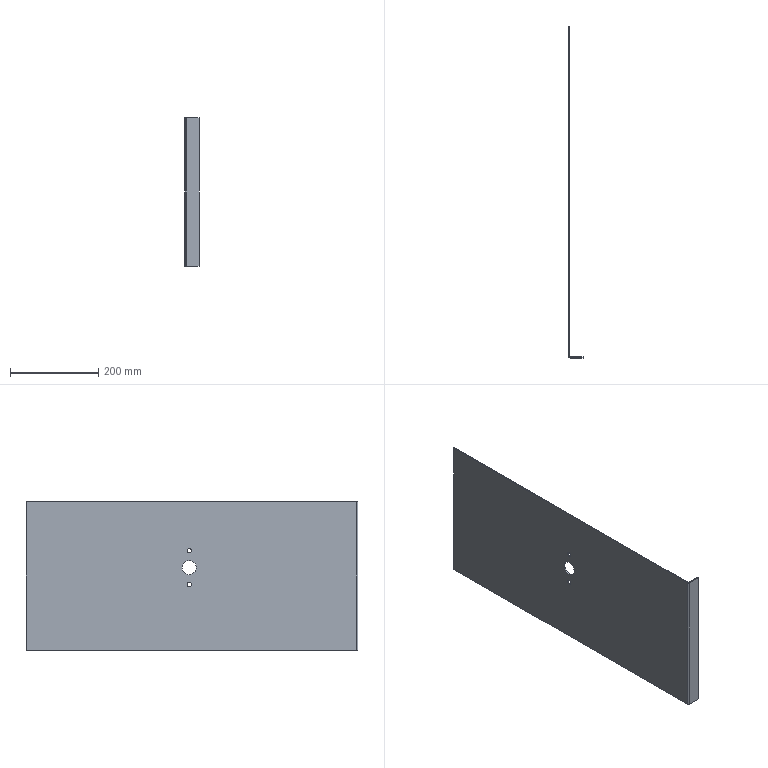Part | SolidWorks | features FlatPattern 1, ICE 1, SMBaseFlange 1, SheetMetal 1 | 1 solid | 20 faces | box 32 x 752 x 337 mm | volume 524643 mm3 | plane 12 | cylinder 8 | commonest cylinder face diameters 10 x4 32 x2 1.473 x1 5.473 x1
STEP:
#1=CARTESIAN_POINT('',(0.,107.626,-14.25));
#2=VERTEX_POINT('',#1);
#3=CARTESIAN_POINT('',(0.,107.626,-24.25));
#4=VERTEX_POINT('',#3);
#5=CARTESIAN_POINT('',(0.,107.626,-19.25));
#6=DIRECTION('',(1.,0.,0.));
#7=DIRECTION('',(0.,0.,-1.));
#8=AXIS2_PLACEMENT_3D('',#5,#6,#7);
#9=CIRCLE('',#8,5.);
#10=EDGE_CURVE('',#2,#4,#9,.T.);
#11=ORIENTED_EDGE('',*,*,#10,.T.);
#12=CARTESIAN_POINT('',(-2.,107.626,-24.25));
#13=VERTEX_POINT('',#12);
#14=CARTESIAN_POINT('',(8.,107.626,-24.25));
#15=DIRECTION('',(-1.,0.,0.));
#16=VECTOR('',#15,1000.);
#17=LINE('',#14,#16);
#18=EDGE_CURVE('',#4,#13,#17,.T.);
#19=ORIENTED_EDGE('',*,*,#18,.T.);
#20=CARTESIAN_POINT('',(-2.,107.626,-14.25));
#21=VERTEX_POINT('',#20);
#22=CARTESIAN_POINT('',(-2.,107.626,-19.25));
#23=DIRECTION('',(-1.,0.,0.));
#24=DIRECTION('',(0.,0.,1.));
#25=AXIS2_PLACEMENT_3D('',#22,#23,#24);
#26=CIRCLE('',#25,5.);
#27=EDGE_CURVE('',#13,#21,#26,.T.);
#28=ORIENTED_EDGE('',*,*,#27,.T.);
#29=CARTESIAN_POINT('',(8.,107.626,-14.25));
#30=DIRECTION('',(-1.,0.,0.));
#31=VECTOR('',#30,1000.);
#32=LINE('',#29,#31);
#33=EDGE_CURVE('',#2,#21,#32,.T.);
#34=ORIENTED_EDGE('',*,*,#33,.F.);
#35=EDGE_LOOP('',(#11,#19,#28,#34));
#36=FACE_OUTER_BOUND('',#35,.T.);
#37=CARTESIAN_POINT('',(8.,107.626,-19.25));
#38=DIRECTION('',(-1.,0.,0.));
#39=DIRECTION('',(0.,0.,1.));
#40=AXIS2_PLACEMENT_3D('',#37,#38,#39);
#41=CYLINDRICAL_SURFACE('',#40,5.);
#42=ADVANCED_FACE('',(#36),#41,.F.);
#43=CARTESIAN_POINT('',(0.,107.626,62.25));
#44=VERTEX_POINT('',#43);
#45=CARTESIAN_POINT('',(0.,107.626,52.25));
#46=VERTEX_POINT('',#45);
#47=CARTESIAN_POINT('',(0.,107.626,57.25));
#48=DIRECTION('',(1.,0.,0.));
#49=DIRECTION('',(0.,0.,-1.));
#50=AXIS2_PLACEMENT_3D('',#47,#48,#49);
#51=CIRCLE('',#50,5.);
#52=EDGE_CURVE('',#44,#46,#51,.T.);
#53=ORIENTED_EDGE('',*,*,#52,.T.);
#54=CARTESIAN_POINT('',(-2.,107.626,52.25));
#55=VERTEX_POINT('',#54);
#56=CARTESIAN_POINT('',(8.,107.626,52.25));
#57=DIRECTION('',(-1.,0.,0.));
#58=VECTOR('',#57,1000.);
#59=LINE('',#56,#58);
#60=EDGE_CURVE('',#46,#55,#59,.T.);
#61=ORIENTED_EDGE('',*,*,#60,.T.);
#62=CARTESIAN_POINT('',(-2.,107.626,62.25));
#63=VERTEX_POINT('',#62);
#64=CARTESIAN_POINT('',(-2.,107.626,57.25));
#65=DIRECTION('',(-1.,0.,0.));
#66=DIRECTION('',(0.,0.,1.));
#67=AXIS2_PLACEMENT_3D('',#64,#65,#66);
#68=CIRCLE('',#67,5.);
#69=EDGE_CURVE('',#55,#63,#68,.T.);
#70=ORIENTED_EDGE('',*,*,#69,.T.);
#71=CARTESIAN_POINT('',(8.,107.626,62.25));
#72=DIRECTION('',(-1.,0.,0.));
#73=VECTOR('',#72,1000.);
#74=LINE('',#71,#73);
#75=EDGE_CURVE('',#44,#63,#74,.T.);
#76=ORIENTED_EDGE('',*,*,#75,.F.);
#77=EDGE_LOOP('',(#53,#61,#70,#76));
#78=FACE_OUTER_BOUND('',#77,.T.);
#79=CARTESIAN_POINT('',(8.,107.626,57.25));
#80=DIRECTION('',(-1.,0.,0.));
#81=DIRECTION('',(0.,0.,1.));
#82=AXIS2_PLACEMENT_3D('',#79,#80,#81);
#83=CYLINDRICAL_SURFACE('',#82,5.);
#84=ADVANCED_FACE('',(#78),#83,.F.);
#85=CARTESIAN_POINT('',(0.,107.626,35.));
#86=VERTEX_POINT('',#85);
#87=CARTESIAN_POINT('',(0.,107.626,3.));
#88=VERTEX_POINT('',#87);
#89=CARTESIAN_POINT('',(0.,107.626,19.));
#90=DIRECTION('',(1.,0.,0.));
#91=DIRECTION('',(0.,0.,-1.));
#92=AXIS2_PLACEMENT_3D('',#89,#90,#91);
#93=CIRCLE('',#92,16.);
#94=EDGE_CURVE('',#86,#88,#93,.T.);
#95=ORIENTED_EDGE('',*,*,#94,.T.);
#96=CARTESIAN_POINT('',(-2.,107.626,3.));
#97=VERTEX_POINT('',#96);
#98=CARTESIAN_POINT('',(8.,107.626,3.));
#99=DIRECTION('',(-1.,0.,0.));
#100=VECTOR('',#99,1000.);
#101=LINE('',#98,#100);
#102=EDGE_CURVE('',#88,#97,#101,.T.);
#103=ORIENTED_EDGE('',*,*,#102,.T.);
#104=CARTESIAN_POINT('',(-2.,107.626,35.));
#105=VERTEX_POINT('',#104);
#106=CARTESIAN_POINT('',(-2.,107.626,19.));
#107=DIRECTION('',(-1.,0.,0.));
#108=DIRECTION('',(0.,0.,1.));
#109=AXIS2_PLACEMENT_3D('',#106,#107,#108);
#110=CIRCLE('',#109,16.);
#111=EDGE_CURVE('',#97,#105,#110,.T.);
#112=ORIENTED_EDGE('',*,*,#111,.T.);
#113=CARTESIAN_POINT('',(8.,107.626,35.));
#114=DIRECTION('',(-1.,0.,0.));
#115=VECTOR('',#114,1000.);
#116=LINE('',#113,#115);
#117=EDGE_CURVE('',#86,#105,#116,.T.);
#118=ORIENTED_EDGE('',*,*,#117,.F.);
#119=EDGE_LOOP('',(#95,#103,#112,#118));
#120=FACE_OUTER_BOUND('',#119,.T.);
#121=CARTESIAN_POINT('',(8.,107.626,19.));
#122=DIRECTION('',(-1.,0.,0.));
#123=DIRECTION('',(0.,0.,1.));
#124=AXIS2_PLACEMENT_3D('',#121,#122,#123);
#125=CYLINDRICAL_SURFACE('',#124,16.);
#126=ADVANCED_FACE('',(#120),#125,.F.);
#127=CARTESIAN_POINT('',(0.7366,-272.664,168.5));
#128=VERTEX_POINT('',#127);
#129=CARTESIAN_POINT('',(0.7366,-274.664,168.5));
#130=VERTEX_POINT('',#129);
#131=CARTESIAN_POINT('',(0.7366,-272.664,168.5));
#132=DIRECTION('',(0.,-1.,0.));
#133=VECTOR('',#132,1000.);
#134=LINE('',#131,#133);
#135=EDGE_CURVE('',#128,#130,#134,.T.);
#136=ORIENTED_EDGE('',*,*,#135,.F.);
#137=CARTESIAN_POINT('',(0.,-271.928,168.5));
#138=VERTEX_POINT('',#137);
#139=CARTESIAN_POINT('',(0.7366,-271.928,168.5));
#140=DIRECTION('',(0.,0.,1.));
#141=DIRECTION('',(-1.,0.,0.));
#142=AXIS2_PLACEMENT_3D('',#139,#140,#141);
#143=CIRCLE('',#142,0.7366);
#144=EDGE_CURVE('',#138,#128,#143,.T.);
#145=ORIENTED_EDGE('',*,*,#144,.F.);
#146=CARTESIAN_POINT('',(-2.,-271.928,168.5));
#147=VERTEX_POINT('',#146);
#148=CARTESIAN_POINT('',(-2.,-271.928,168.5));
#149=DIRECTION('',(1.,0.,0.));
#150=VECTOR('',#149,1000.);
#151=LINE('',#148,#150);
#152=EDGE_CURVE('',#147,#138,#151,.T.);
#153=ORIENTED_EDGE('',*,*,#152,.F.);
#154=CARTESIAN_POINT('',(0.7366,-271.928,168.5));
#155=DIRECTION('',(0.,0.,1.));
#156=DIRECTION('',(1.,0.,0.));
#157=AXIS2_PLACEMENT_3D('',#154,#155,#156);
#158=CIRCLE('',#157,2.737);
#159=EDGE_CURVE('',#147,#130,#158,.T.);
#160=ORIENTED_EDGE('',*,*,#159,.T.);
#161=EDGE_LOOP('',(#136,#145,#153,#160));
#162=FACE_OUTER_BOUND('',#161,.T.);
#163=CARTESIAN_POINT('',(0.7366,-272.664,168.5));
#164=DIRECTION('',(0.,0.,1.));
#165=DIRECTION('',(1.,0.,0.));
#166=AXIS2_PLACEMENT_3D('',#163,#164,#165);
#167=PLANE('',#166);
#168=ADVANCED_FACE('',(#162),#167,.T.);
#169=CARTESIAN_POINT('',(30.,-272.664,168.5));
#170=VERTEX_POINT('',#169);
#171=CARTESIAN_POINT('',(0.,-272.664,168.5));
#172=DIRECTION('',(1.,0.,0.));
#173=VECTOR('',#172,1000.);
#174=LINE('',#171,#173);
#175=EDGE_CURVE('',#128,#170,#174,.T.);
#176=ORIENTED_EDGE('',*,*,#175,.F.);
#177=ORIENTED_EDGE('',*,*,#135,.T.);
#178=CARTESIAN_POINT('',(30.,-274.664,168.5));
#179=VERTEX_POINT('',#178);
#180=CARTESIAN_POINT('',(0.,-274.664,168.5));
#181=DIRECTION('',(1.,0.,0.));
#182=VECTOR('',#181,1000.);
#183=LINE('',#180,#182);
#184=EDGE_CURVE('',#130,#179,#183,.T.);
#185=ORIENTED_EDGE('',*,*,#184,.T.);
#186=CARTESIAN_POINT('',(30.,-272.664,168.5));
#187=DIRECTION('',(0.,-1.,0.));
#188=VECTOR('',#187,1000.);
#189=LINE('',#186,#188);
#190=EDGE_CURVE('',#170,#179,#189,.T.);
#191=ORIENTED_EDGE('',*,*,#190,.F.);
#192=EDGE_LOOP('',(#176,#177,#185,#191));
#193=FACE_OUTER_BOUND('',#192,.T.);
#194=CARTESIAN_POINT('',(-2.,-271.928,168.5));
#195=DIRECTION('',(0.,0.,1.));
#196=DIRECTION('',(1.,0.,0.));
#197=AXIS2_PLACEMENT_3D('',#194,#195,#196);
#198=PLANE('',#197);
#199=ADVANCED_FACE('',(#193),#198,.T.);
#200=CARTESIAN_POINT('',(0.,-271.928,-168.5));
#201=VERTEX_POINT('',#200);
#202=CARTESIAN_POINT('',(-2.,-271.928,-168.5));
#203=VERTEX_POINT('',#202);
#204=CARTESIAN_POINT('',(0.,-271.928,-168.5));
#205=DIRECTION('',(-1.,0.,0.));
#206=VECTOR('',#205,1000.);
#207=LINE('',#204,#206);
#208=EDGE_CURVE('',#201,#203,#207,.T.);
#209=ORIENTED_EDGE('',*,*,#208,.F.);
#210=CARTESIAN_POINT('',(0.7366,-272.664,-168.5));
#211=VERTEX_POINT('',#210);
#212=CARTESIAN_POINT('',(0.7366,-271.928,-168.5));
#213=DIRECTION('',(0.,0.,1.));
#214=DIRECTION('',(-1.,0.,0.));
#215=AXIS2_PLACEMENT_3D('',#212,#213,#214);
#216=CIRCLE('',#215,0.7366);
#217=EDGE_CURVE('',#201,#211,#216,.T.);
#218=ORIENTED_EDGE('',*,*,#217,.T.);
#219=CARTESIAN_POINT('',(0.7366,-274.664,-168.5));
#220=VERTEX_POINT('',#219);
#221=CARTESIAN_POINT('',(0.7366,-274.664,-168.5));
#222=DIRECTION('',(0.,1.,0.));
#223=VECTOR('',#222,1000.);
#224=LINE('',#221,#223);
#225=EDGE_CURVE('',#220,#211,#224,.T.);
#226=ORIENTED_EDGE('',*,*,#225,.F.);
#227=CARTESIAN_POINT('',(0.7366,-271.928,-168.5));
#228=DIRECTION('',(0.,0.,1.));
#229=DIRECTION('',(1.,0.,0.));
#230=AXIS2_PLACEMENT_3D('',#227,#228,#229);
#231=CIRCLE('',#230,2.737);
#232=EDGE_CURVE('',#203,#220,#231,.T.);
#233=ORIENTED_EDGE('',*,*,#232,.F.);
#234=EDGE_LOOP('',(#209,#218,#226,#233));
#235=FACE_OUTER_BOUND('',#234,.T.);
#236=CARTESIAN_POINT('',(0.,-271.928,-168.5));
#237=DIRECTION('',(0.,0.,-1.));
#238=DIRECTION('',(-1.,0.,0.));
#239=AXIS2_PLACEMENT_3D('',#236,#237,#238);
#240=PLANE('',#239);
#241=ADVANCED_FACE('',(#235),#240,.T.);
#242=CARTESIAN_POINT('',(0.,477.336,-168.5));
#243=VERTEX_POINT('',#242);
#244=CARTESIAN_POINT('',(0.,477.336,-168.5));
#245=DIRECTION('',(0.,-1.,0.));
#246=VECTOR('',#245,1000.);
#247=LINE('',#244,#246);
#248=EDGE_CURVE('',#243,#201,#247,.T.);
#249=ORIENTED_EDGE('',*,*,#248,.T.);
#250=ORIENTED_EDGE('',*,*,#208,.T.);
#251=CARTESIAN_POINT('',(-2.,477.336,-168.5));
#252=VERTEX_POINT('',#251);
#253=CARTESIAN_POINT('',(-2.,477.336,-168.5));
#254=DIRECTION('',(0.,-1.,0.));
#255=VECTOR('',#254,1000.);
#256=LINE('',#253,#255);
#257=EDGE_CURVE('',#252,#203,#256,.T.);
#258=ORIENTED_EDGE('',*,*,#257,.F.);
#259=CARTESIAN_POINT('',(-2.,477.336,-168.5));
#260=DIRECTION('',(1.,0.,0.));
#261=VECTOR('',#260,1000.);
#262=LINE('',#259,#261);
#263=EDGE_CURVE('',#252,#243,#262,.T.);
#264=ORIENTED_EDGE('',*,*,#263,.T.);
#265=EDGE_LOOP('',(#249,#250,#258,#264));
#266=FACE_OUTER_BOUND('',#265,.T.);
#267=CARTESIAN_POINT('',(0.7366,-274.664,-168.5));
#268=DIRECTION('',(0.,0.,-1.));
#269=DIRECTION('',(-1.,0.,0.));
#270=AXIS2_PLACEMENT_3D('',#267,#268,#269);
#271=PLANE('',#270);
#272=ADVANCED_FACE('',(#266),#271,.T.);
#273=CARTESIAN_POINT('',(30.,-274.664,-168.5));
#274=VERTEX_POINT('',#273);
#275=CARTESIAN_POINT('',(0.,-274.664,-168.5));
#276=DIRECTION('',(1.,0.,0.));
#277=VECTOR('',#276,1000.);
#278=LINE('',#275,#277);
#279=EDGE_CURVE('',#220,#274,#278,.T.);
#280=ORIENTED_EDGE('',*,*,#279,.T.);
#281=CARTESIAN_POINT('',(30.,-274.664,168.5));
#282=DIRECTION('',(0.,0.,-1.));
#283=VECTOR('',#282,1000.);
#284=LINE('',#281,#283);
#285=EDGE_CURVE('',#179,#274,#284,.T.);
#286=ORIENTED_EDGE('',*,*,#285,.F.);
#287=ORIENTED_EDGE('',*,*,#184,.F.);
#288=CARTESIAN_POINT('',(0.7366,-274.664,168.5));
#289=DIRECTION('',(0.,0.,-1.));
#290=VECTOR('',#289,1000.);
#291=LINE('',#288,#290);
#292=EDGE_CURVE('',#130,#220,#291,.T.);
#293=ORIENTED_EDGE('',*,*,#292,.T.);
#294=EDGE_LOOP('',(#280,#286,#287,#293));
#295=FACE_OUTER_BOUND('',#294,.T.);
#296=CARTESIAN_POINT('',(0.,-274.664,168.5));
#297=DIRECTION('',(0.,1.,0.));
#298=DIRECTION('',(0.,0.,1.));
#299=AXIS2_PLACEMENT_3D('',#296,#297,#298);
#300=PLANE('',#299);
#301=ADVANCED_FACE('',(#295),#300,.F.);
#302=CARTESIAN_POINT('',(30.,-272.664,-168.5));
#303=VERTEX_POINT('',#302);
#304=CARTESIAN_POINT('',(30.,-272.664,-168.5));
#305=DIRECTION('',(0.,-1.,0.));
#306=VECTOR('',#305,1000.);
#307=LINE('',#304,#306);
#308=EDGE_CURVE('',#303,#274,#307,.T.);
#309=ORIENTED_EDGE('',*,*,#308,.F.);
#310=CARTESIAN_POINT('',(30.,-272.664,168.5));
#311=DIRECTION('',(0.,0.,-1.));
#312=VECTOR('',#311,1000.);
#313=LINE('',#310,#312);
#314=EDGE_CURVE('',#170,#303,#313,.T.);
#315=ORIENTED_EDGE('',*,*,#314,.F.);
#316=ORIENTED_EDGE('',*,*,#190,.T.);
#317=ORIENTED_EDGE('',*,*,#285,.T.);
#318=EDGE_LOOP('',(#309,#315,#316,#317));
#319=FACE_OUTER_BOUND('',#318,.T.);
#320=CARTESIAN_POINT('',(30.,-272.664,168.5));
#321=DIRECTION('',(1.,0.,0.));
#322=DIRECTION('',(0.,0.,-1.));
#323=AXIS2_PLACEMENT_3D('',#320,#321,#322);
#324=PLANE('',#323);
#325=ADVANCED_FACE('',(#319),#324,.T.);
#326=CARTESIAN_POINT('',(0.,-272.664,-168.5));
#327=DIRECTION('',(1.,0.,0.));
#328=VECTOR('',#327,1000.);
#329=LINE('',#326,#328);
#330=EDGE_CURVE('',#211,#303,#329,.T.);
#331=ORIENTED_EDGE('',*,*,#330,.F.);
#332=CARTESIAN_POINT('',(0.7366,-272.664,168.5));
#333=DIRECTION('',(0.,0.,-1.));
#334=VECTOR('',#333,1000.);
#335=LINE('',#332,#334);
#336=EDGE_CURVE('',#128,#211,#335,.T.);
#337=ORIENTED_EDGE('',*,*,#336,.F.);
#338=ORIENTED_EDGE('',*,*,#175,.T.);
#339=ORIENTED_EDGE('',*,*,#314,.T.);
#340=EDGE_LOOP('',(#331,#337,#338,#339));
#341=FACE_OUTER_BOUND('',#340,.T.);
#342=CARTESIAN_POINT('',(0.,-272.664,168.5));
#343=DIRECTION('',(0.,1.,0.));
#344=DIRECTION('',(0.,0.,1.));
#345=AXIS2_PLACEMENT_3D('',#342,#343,#344);
#346=PLANE('',#345);
#347=ADVANCED_FACE('',(#341),#346,.T.);
#348=ORIENTED_EDGE('',*,*,#217,.F.);
#349=CARTESIAN_POINT('',(0.,-271.928,168.5));
#350=DIRECTION('',(0.,0.,-1.));
#351=VECTOR('',#350,1000.);
#352=LINE('',#349,#351);
#353=EDGE_CURVE('',#138,#201,#352,.T.);
#354=ORIENTED_EDGE('',*,*,#353,.F.);
#355=ORIENTED_EDGE('',*,*,#144,.T.);
#356=ORIENTED_EDGE('',*,*,#336,.T.);
#357=EDGE_LOOP('',(#348,#354,#355,#356));
#358=FACE_OUTER_BOUND('',#357,.T.);
#359=CARTESIAN_POINT('',(0.7366,-271.928,168.5));
#360=DIRECTION('',(0.,0.,-1.));
#361=DIRECTION('',(-1.,0.,0.));
#362=AXIS2_PLACEMENT_3D('',#359,#360,#361);
#363=CYLINDRICAL_SURFACE('',#362,0.7366);
#364=ADVANCED_FACE('',(#358),#363,.F.);
#365=ORIENTED_EDGE('',*,*,#10,.F.);
#366=CARTESIAN_POINT('',(0.,107.626,-19.25));
#367=DIRECTION('',(1.,0.,0.));
#368=DIRECTION('',(0.,0.,-1.));
#369=AXIS2_PLACEMENT_3D('',#366,#367,#368);
#370=CIRCLE('',#369,5.);
#371=EDGE_CURVE('',#4,#2,#370,.T.);
#372=ORIENTED_EDGE('',*,*,#371,.F.);
#373=EDGE_LOOP('',(#365,#372));
#374=FACE_BOUND('',#373,.T.);
#375=ORIENTED_EDGE('',*,*,#52,.F.);
#376=CARTESIAN_POINT('',(0.,107.626,57.25));
#377=DIRECTION('',(1.,0.,0.));
#378=DIRECTION('',(0.,0.,-1.));
#379=AXIS2_PLACEMENT_3D('',#376,#377,#378);
#380=CIRCLE('',#379,5.);
#381=EDGE_CURVE('',#46,#44,#380,.T.);
#382=ORIENTED_EDGE('',*,*,#381,.F.);
#383=EDGE_LOOP('',(#375,#382));
#384=FACE_BOUND('',#383,.T.);
#385=ORIENTED_EDGE('',*,*,#94,.F.);
#386=CARTESIAN_POINT('',(0.,107.626,19.));
#387=DIRECTION('',(1.,0.,0.));
#388=DIRECTION('',(0.,0.,-1.));
#389=AXIS2_PLACEMENT_3D('',#386,#387,#388);
#390=CIRCLE('',#389,16.);
#391=EDGE_CURVE('',#88,#86,#390,.T.);
#392=ORIENTED_EDGE('',*,*,#391,.F.);
#393=EDGE_LOOP('',(#385,#392));
#394=FACE_BOUND('',#393,.T.);
#395=ORIENTED_EDGE('',*,*,#248,.F.);
#396=CARTESIAN_POINT('',(0.,477.336,168.5));
#397=VERTEX_POINT('',#396);
#398=CARTESIAN_POINT('',(0.,477.336,168.5));
#399=DIRECTION('',(0.,0.,-1.));
#400=VECTOR('',#399,1000.);
#401=LINE('',#398,#400);
#402=EDGE_CURVE('',#397,#243,#401,.T.);
#403=ORIENTED_EDGE('',*,*,#402,.F.);
#404=CARTESIAN_POINT('',(0.,477.336,168.5));
#405=DIRECTION('',(0.,-1.,0.));
#406=VECTOR('',#405,1000.);
#407=LINE('',#404,#406);
#408=EDGE_CURVE('',#397,#138,#407,.T.);
#409=ORIENTED_EDGE('',*,*,#408,.T.);
#410=ORIENTED_EDGE('',*,*,#353,.T.);
#411=EDGE_LOOP('',(#395,#403,#409,#410));
#412=FACE_OUTER_BOUND('',#411,.T.);
#413=CARTESIAN_POINT('',(0.,477.336,168.5));
#414=DIRECTION('',(1.,0.,0.));
#415=DIRECTION('',(0.,0.,-1.));
#416=AXIS2_PLACEMENT_3D('',#413,#414,#415);
#417=PLANE('',#416);
#418=ADVANCED_FACE('',(#374,#384,#394,#412),#417,.T.);
#419=ORIENTED_EDGE('',*,*,#263,.F.);
#420=CARTESIAN_POINT('',(-2.,477.336,168.5));
#421=VERTEX_POINT('',#420);
#422=CARTESIAN_POINT('',(-2.,477.336,168.5));
#423=DIRECTION('',(0.,0.,-1.));
#424=VECTOR('',#423,1000.);
#425=LINE('',#422,#424);
#426=EDGE_CURVE('',#421,#252,#425,.T.);
#427=ORIENTED_EDGE('',*,*,#426,.F.);
#428=CARTESIAN_POINT('',(-2.,477.336,168.5));
#429=DIRECTION('',(1.,0.,0.));
#430=VECTOR('',#429,1000.);
#431=LINE('',#428,#430);
#432=EDGE_CURVE('',#421,#397,#431,.T.);
#433=ORIENTED_EDGE('',*,*,#432,.T.);
#434=ORIENTED_EDGE('',*,*,#402,.T.);
#435=EDGE_LOOP('',(#419,#427,#433,#434));
#436=FACE_OUTER_BOUND('',#435,.T.);
#437=CARTESIAN_POINT('',(-2.,477.336,168.5));
#438=DIRECTION('',(0.,1.,0.));
#439=DIRECTION('',(0.,0.,1.));
#440=AXIS2_PLACEMENT_3D('',#437,#438,#439);
#441=PLANE('',#440);
#442=ADVANCED_FACE('',(#436),#441,.T.);
#443=CARTESIAN_POINT('',(-2.,107.626,-19.25));
#444=DIRECTION('',(-1.,0.,0.));
#445=DIRECTION('',(0.,0.,1.));
#446=AXIS2_PLACEMENT_3D('',#443,#444,#445);
#447=CIRCLE('',#446,5.);
#448=EDGE_CURVE('',#21,#13,#447,.T.);
#449=ORIENTED_EDGE('',*,*,#448,.F.);
#450=ORIENTED_EDGE('',*,*,#27,.F.);
#451=EDGE_LOOP('',(#449,#450));
#452=FACE_BOUND('',#451,.T.);
#453=CARTESIAN_POINT('',(-2.,107.626,57.25));
#454=DIRECTION('',(-1.,0.,0.));
#455=DIRECTION('',(0.,0.,1.));
#456=AXIS2_PLACEMENT_3D('',#453,#454,#455);
#457=CIRCLE('',#456,5.);
#458=EDGE_CURVE('',#63,#55,#457,.T.);
#459=ORIENTED_EDGE('',*,*,#458,.F.);
#460=ORIENTED_EDGE('',*,*,#69,.F.);
#461=EDGE_LOOP('',(#459,#460));
#462=FACE_BOUND('',#461,.T.);
#463=CARTESIAN_POINT('',(-2.,107.626,19.));
#464=DIRECTION('',(-1.,0.,0.));
#465=DIRECTION('',(0.,0.,1.));
#466=AXIS2_PLACEMENT_3D('',#463,#464,#465);
#467=CIRCLE('',#466,16.);
#468=EDGE_CURVE('',#105,#97,#467,.T.);
#469=ORIENTED_EDGE('',*,*,#468,.F.);
#470=ORIENTED_EDGE('',*,*,#111,.F.);
#471=EDGE_LOOP('',(#469,#470));
#472=FACE_BOUND('',#471,.T.);
#473=ORIENTED_EDGE('',*,*,#257,.T.);
#474=CARTESIAN_POINT('',(-2.,-271.928,168.5));
#475=DIRECTION('',(0.,0.,-1.));
#476=VECTOR('',#475,1000.);
#477=LINE('',#474,#476);
#478=EDGE_CURVE('',#147,#203,#477,.T.);
#479=ORIENTED_EDGE('',*,*,#478,.F.);
#480=CARTESIAN_POINT('',(-2.,477.336,168.5));
#481=DIRECTION('',(0.,-1.,0.));
#482=VECTOR('',#481,1000.);
#483=LINE('',#480,#482);
#484=EDGE_CURVE('',#421,#147,#483,.T.);
#485=ORIENTED_EDGE('',*,*,#484,.F.);
#486=ORIENTED_EDGE('',*,*,#426,.T.);
#487=EDGE_LOOP('',(#473,#479,#485,#486));
#488=FACE_OUTER_BOUND('',#487,.T.);
#489=CARTESIAN_POINT('',(-2.,477.336,168.5));
#490=DIRECTION('',(1.,0.,0.));
#491=DIRECTION('',(0.,0.,-1.));
#492=AXIS2_PLACEMENT_3D('',#489,#490,#491);
#493=PLANE('',#492);
#494=ADVANCED_FACE('',(#452,#462,#472,#488),#493,.F.);
#495=ORIENTED_EDGE('',*,*,#232,.T.);
#496=ORIENTED_EDGE('',*,*,#292,.F.);
#497=ORIENTED_EDGE('',*,*,#159,.F.);
#498=ORIENTED_EDGE('',*,*,#478,.T.);
#499=EDGE_LOOP('',(#495,#496,#497,#498));
#500=FACE_OUTER_BOUND('',#499,.T.);
#501=CARTESIAN_POINT('',(0.7366,-271.928,168.5));
#502=DIRECTION('',(0.,0.,-1.));
#503=DIRECTION('',(-1.,0.,0.));
#504=AXIS2_PLACEMENT_3D('',#501,#502,#503);
#505=CYLINDRICAL_SURFACE('',#504,2.737);
#506=ADVANCED_FACE('',(#500),#505,.T.);
#507=ORIENTED_EDGE('',*,*,#484,.T.);
#508=ORIENTED_EDGE('',*,*,#152,.T.);
#509=ORIENTED_EDGE('',*,*,#408,.F.);
#510=ORIENTED_EDGE('',*,*,#432,.F.);
#511=EDGE_LOOP('',(#507,#508,#509,#510));
#512=FACE_OUTER_BOUND('',#511,.T.);
#513=CARTESIAN_POINT('',(0.7366,-271.928,168.5));
#514=DIRECTION('',(0.,0.,-1.));
#515=DIRECTION('',(-1.,0.,0.));
#516=AXIS2_PLACEMENT_3D('',#513,#514,#515);
#517=PLANE('',#516);
#518=ADVANCED_FACE('',(#512),#517,.F.);
#519=ORIENTED_EDGE('',*,*,#279,.F.);
#520=ORIENTED_EDGE('',*,*,#225,.T.);
#521=ORIENTED_EDGE('',*,*,#330,.T.);
#522=ORIENTED_EDGE('',*,*,#308,.T.);
#523=EDGE_LOOP('',(#519,#520,#521,#522));
#524=FACE_OUTER_BOUND('',#523,.T.);
#525=CARTESIAN_POINT('',(0.7366,-271.928,-168.5));
#526=DIRECTION('',(0.,0.,-1.));
#527=DIRECTION('',(-1.,0.,0.));
#528=AXIS2_PLACEMENT_3D('',#525,#526,#527);
#529=PLANE('',#528);
#530=ADVANCED_FACE('',(#524),#529,.T.);
#531=ORIENTED_EDGE('',*,*,#102,.F.);
#532=ORIENTED_EDGE('',*,*,#391,.T.);
#533=ORIENTED_EDGE('',*,*,#117,.T.);
#534=ORIENTED_EDGE('',*,*,#468,.T.);
#535=EDGE_LOOP('',(#531,#532,#533,#534));
#536=FACE_OUTER_BOUND('',#535,.T.);
#537=CARTESIAN_POINT('',(8.,107.626,19.));
#538=DIRECTION('',(-1.,0.,0.));
#539=DIRECTION('',(0.,0.,1.));
#540=AXIS2_PLACEMENT_3D('',#537,#538,#539);
#541=CYLINDRICAL_SURFACE('',#540,16.);
#542=ADVANCED_FACE('',(#536),#541,.F.);
#543=ORIENTED_EDGE('',*,*,#60,.F.);
#544=ORIENTED_EDGE('',*,*,#381,.T.);
#545=ORIENTED_EDGE('',*,*,#75,.T.);
#546=ORIENTED_EDGE('',*,*,#458,.T.);
#547=EDGE_LOOP('',(#543,#544,#545,#546));
#548=FACE_OUTER_BOUND('',#547,.T.);
#549=CARTESIAN_POINT('',(8.,107.626,57.25));
#550=DIRECTION('',(-1.,0.,0.));
#551=DIRECTION('',(0.,0.,1.));
#552=AXIS2_PLACEMENT_3D('',#549,#550,#551);
#553=CYLINDRICAL_SURFACE('',#552,5.);
#554=ADVANCED_FACE('',(#548),#553,.F.);
#555=ORIENTED_EDGE('',*,*,#18,.F.);
#556=ORIENTED_EDGE('',*,*,#371,.T.);
#557=ORIENTED_EDGE('',*,*,#33,.T.);
#558=ORIENTED_EDGE('',*,*,#448,.T.);
#559=EDGE_LOOP('',(#555,#556,#557,#558));
#560=FACE_OUTER_BOUND('',#559,.T.);
#561=CARTESIAN_POINT('',(8.,107.626,-19.25));
#562=DIRECTION('',(-1.,0.,0.));
#563=DIRECTION('',(0.,0.,1.));
#564=AXIS2_PLACEMENT_3D('',#561,#562,#563);
#565=CYLINDRICAL_SURFACE('',#564,5.);
#566=ADVANCED_FACE('',(#560),#565,.F.);
#567=CLOSED_SHELL('',(#42,#84,#126,#168,#199,#241,#272,#301,#325,#347,#364,#418,#442,#494,#506,#518,#530,#542,#554,#566));
#568=MANIFOLD_SOLID_BREP('',#567);
#569=CARTESIAN_POINT('',(0.,0.,0.));
#570=DIRECTION('',(0.,0.,1.));
#571=DIRECTION('',(1.,0.,0.));
#572=AXIS2_PLACEMENT_3D('',#569,#570,#571);
#573=(LENGTH_UNIT()NAMED_UNIT(*)SI_UNIT(.MILLI.,.METRE.));
#574=UNCERTAINTY_MEASURE_WITH_UNIT(LENGTH_MEASURE(0.00001),#573,'','');
#575=(NAMED_UNIT(*)PLANE_ANGLE_UNIT()SI_UNIT($,.RADIAN.));
#576=(NAMED_UNIT(*)SI_UNIT($,.STERADIAN.)SOLID_ANGLE_UNIT());
#577=(GEOMETRIC_REPRESENTATION_CONTEXT(3)GLOBAL_UNCERTAINTY_ASSIGNED_CONTEXT((#574))GLOBAL_UNIT_ASSIGNED_CONTEXT((#573,#575,#576))REPRESENTATION_CONTEXT('',''));
#578=ADVANCED_BREP_SHAPE_REPRESENTATION('',(#568,#572),#577);